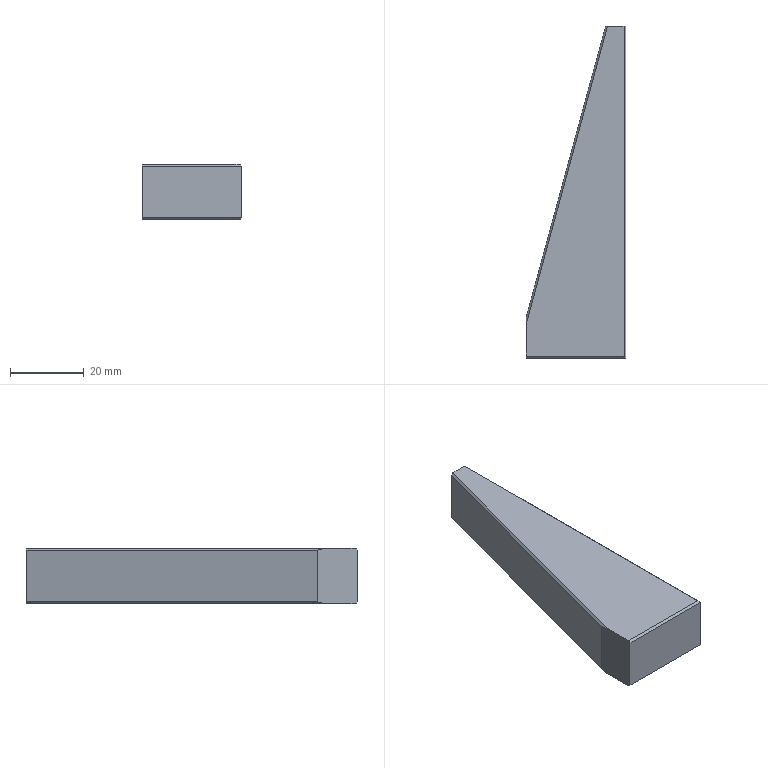Part | SolidWorks | features Chamfer 1, Extrusion 1, ICE 1 | 1 solid | 13 faces | box 27 x 89.833 x 15 mm | volume 23621 mm3 | plane 13
STEP:
#1=CARTESIAN_POINT('',(24.5,89.833,0.5));
#2=VERTEX_POINT('',#1);
#3=CARTESIAN_POINT('',(3.,11.,0.5));
#4=VERTEX_POINT('',#3);
#5=CARTESIAN_POINT('',(30.,110.,0.5));
#6=DIRECTION('',(-0.2631,-0.9648,0.));
#7=VECTOR('',#6,1000.);
#8=LINE('',#5,#7);
#9=EDGE_CURVE('',#2,#4,#8,.T.);
#10=ORIENTED_EDGE('',*,*,#9,.T.);
#11=CARTESIAN_POINT('',(3.,11.,14.5));
#12=VERTEX_POINT('',#11);
#13=CARTESIAN_POINT('',(3.,11.,15.));
#14=DIRECTION('',(0.,0.,1.));
#15=VECTOR('',#14,1000.);
#16=LINE('',#13,#15);
#17=EDGE_CURVE('',#4,#12,#16,.T.);
#18=ORIENTED_EDGE('',*,*,#17,.T.);
#19=CARTESIAN_POINT('',(24.5,89.833,14.5));
#20=VERTEX_POINT('',#19);
#21=CARTESIAN_POINT('',(30.,110.,14.5));
#22=DIRECTION('',(0.2631,0.9648,0.));
#23=VECTOR('',#22,1000.);
#24=LINE('',#21,#23);
#25=EDGE_CURVE('',#12,#20,#24,.T.);
#26=ORIENTED_EDGE('',*,*,#25,.T.);
#27=CARTESIAN_POINT('',(24.5,89.833,0.));
#28=DIRECTION('',(0.,0.,1.));
#29=VECTOR('',#28,1000.);
#30=LINE('',#27,#29);
#31=EDGE_CURVE('',#2,#20,#30,.T.);
#32=ORIENTED_EDGE('',*,*,#31,.F.);
#33=EDGE_LOOP('',(#10,#18,#26,#32));
#34=FACE_OUTER_BOUND('',#33,.T.);
#35=CARTESIAN_POINT('',(30.,110.,15.));
#36=DIRECTION('',(0.9648,-0.2631,0.));
#37=DIRECTION('',(0.2631,0.9648,0.));
#38=AXIS2_PLACEMENT_3D('',#35,#36,#37);
#39=PLANE('',#38);
#40=ADVANCED_FACE('',(#34),#39,.F.);
#41=CARTESIAN_POINT('',(30.,0.,14.5));
#42=VERTEX_POINT('',#41);
#43=CARTESIAN_POINT('',(3.,0.,14.5));
#44=VERTEX_POINT('',#43);
#45=CARTESIAN_POINT('',(0.,0.,14.5));
#46=DIRECTION('',(-1.,0.,0.));
#47=VECTOR('',#46,1000.);
#48=LINE('',#45,#47);
#49=EDGE_CURVE('',#42,#44,#48,.T.);
#50=ORIENTED_EDGE('',*,*,#49,.T.);
#51=CARTESIAN_POINT('',(3.,0.,0.5));
#52=VERTEX_POINT('',#51);
#53=CARTESIAN_POINT('',(3.,0.,0.));
#54=DIRECTION('',(0.,0.,1.));
#55=VECTOR('',#54,1000.);
#56=LINE('',#53,#55);
#57=EDGE_CURVE('',#52,#44,#56,.T.);
#58=ORIENTED_EDGE('',*,*,#57,.F.);
#59=CARTESIAN_POINT('',(30.,0.,0.5));
#60=VERTEX_POINT('',#59);
#61=CARTESIAN_POINT('',(0.,0.,0.5));
#62=DIRECTION('',(1.,0.,0.));
#63=VECTOR('',#62,1000.);
#64=LINE('',#61,#63);
#65=EDGE_CURVE('',#52,#60,#64,.T.);
#66=ORIENTED_EDGE('',*,*,#65,.T.);
#67=CARTESIAN_POINT('',(30.,0.,15.));
#68=DIRECTION('',(0.,0.,-1.));
#69=VECTOR('',#68,1000.);
#70=LINE('',#67,#69);
#71=EDGE_CURVE('',#42,#60,#70,.T.);
#72=ORIENTED_EDGE('',*,*,#71,.F.);
#73=EDGE_LOOP('',(#50,#58,#66,#72));
#74=FACE_OUTER_BOUND('',#73,.T.);
#75=CARTESIAN_POINT('',(0.,0.,15.));
#76=DIRECTION('',(0.,1.,0.));
#77=DIRECTION('',(0.,0.,1.));
#78=AXIS2_PLACEMENT_3D('',#75,#76,#77);
#79=PLANE('',#78);
#80=ADVANCED_FACE('',(#74),#79,.F.);
#81=CARTESIAN_POINT('',(30.,89.833,0.5));
#82=VERTEX_POINT('',#81);
#83=CARTESIAN_POINT('',(30.,0.,0.5));
#84=DIRECTION('',(0.,1.,0.));
#85=VECTOR('',#84,1000.);
#86=LINE('',#83,#85);
#87=EDGE_CURVE('',#60,#82,#86,.T.);
#88=ORIENTED_EDGE('',*,*,#87,.T.);
#89=CARTESIAN_POINT('',(30.,89.833,14.5));
#90=VERTEX_POINT('',#89);
#91=CARTESIAN_POINT('',(30.,89.833,0.));
#92=DIRECTION('',(0.,0.,1.));
#93=VECTOR('',#92,1000.);
#94=LINE('',#91,#93);
#95=EDGE_CURVE('',#82,#90,#94,.T.);
#96=ORIENTED_EDGE('',*,*,#95,.T.);
#97=CARTESIAN_POINT('',(30.,0.,14.5));
#98=DIRECTION('',(0.,-1.,0.));
#99=VECTOR('',#98,1000.);
#100=LINE('',#97,#99);
#101=EDGE_CURVE('',#90,#42,#100,.T.);
#102=ORIENTED_EDGE('',*,*,#101,.T.);
#103=ORIENTED_EDGE('',*,*,#71,.T.);
#104=EDGE_LOOP('',(#88,#96,#102,#103));
#105=FACE_OUTER_BOUND('',#104,.T.);
#106=CARTESIAN_POINT('',(30.,0.,15.));
#107=DIRECTION('',(-1.,0.,0.));
#108=DIRECTION('',(0.,0.,1.));
#109=AXIS2_PLACEMENT_3D('',#106,#107,#108);
#110=PLANE('',#109);
#111=ADVANCED_FACE('',(#105),#110,.F.);
#112=CARTESIAN_POINT('',(3.,0.5,15.));
#113=VERTEX_POINT('',#112);
#114=CARTESIAN_POINT('',(3.,9.1,15.));
#115=VERTEX_POINT('',#114);
#116=CARTESIAN_POINT('',(3.,0.,15.));
#117=DIRECTION('',(0.,1.,0.));
#118=VECTOR('',#117,1000.);
#119=LINE('',#116,#118);
#120=EDGE_CURVE('',#113,#115,#119,.T.);
#121=ORIENTED_EDGE('',*,*,#120,.F.);
#122=CARTESIAN_POINT('',(29.5,0.5,15.));
#123=VERTEX_POINT('',#122);
#124=CARTESIAN_POINT('',(30.,0.5,15.));
#125=DIRECTION('',(1.,0.,0.));
#126=VECTOR('',#125,1000.);
#127=LINE('',#124,#126);
#128=EDGE_CURVE('',#113,#123,#127,.T.);
#129=ORIENTED_EDGE('',*,*,#128,.T.);
#130=CARTESIAN_POINT('',(29.5,89.833,15.));
#131=VERTEX_POINT('',#130);
#132=CARTESIAN_POINT('',(29.5,110.,15.));
#133=DIRECTION('',(0.,1.,0.));
#134=VECTOR('',#133,1000.);
#135=LINE('',#132,#134);
#136=EDGE_CURVE('',#123,#131,#135,.T.);
#137=ORIENTED_EDGE('',*,*,#136,.T.);
#138=CARTESIAN_POINT('',(25.018,89.833,15.));
#139=VERTEX_POINT('',#138);
#140=CARTESIAN_POINT('',(30.,89.833,15.));
#141=DIRECTION('',(1.,0.,0.));
#142=VECTOR('',#141,1000.);
#143=LINE('',#140,#142);
#144=EDGE_CURVE('',#139,#131,#143,.T.);
#145=ORIENTED_EDGE('',*,*,#144,.F.);
#146=CARTESIAN_POINT('',(0.4824,-0.1316,15.));
#147=DIRECTION('',(-0.2631,-0.9648,0.));
#148=VECTOR('',#147,1000.);
#149=LINE('',#146,#148);
#150=EDGE_CURVE('',#139,#115,#149,.T.);
#151=ORIENTED_EDGE('',*,*,#150,.T.);
#152=EDGE_LOOP('',(#121,#129,#137,#145,#151));
#153=FACE_OUTER_BOUND('',#152,.T.);
#154=CARTESIAN_POINT('',(0.,0.,15.));
#155=DIRECTION('',(0.,0.,1.));
#156=DIRECTION('',(1.,0.,0.));
#157=AXIS2_PLACEMENT_3D('',#154,#155,#156);
#158=PLANE('',#157);
#159=ADVANCED_FACE('',(#153),#158,.T.);
#160=CARTESIAN_POINT('',(29.5,0.5,0.));
#161=VERTEX_POINT('',#160);
#162=CARTESIAN_POINT('',(3.,0.5,0.));
#163=VERTEX_POINT('',#162);
#164=CARTESIAN_POINT('',(0.,0.5,0.));
#165=DIRECTION('',(-1.,0.,0.));
#166=VECTOR('',#165,1000.);
#167=LINE('',#164,#166);
#168=EDGE_CURVE('',#161,#163,#167,.T.);
#169=ORIENTED_EDGE('',*,*,#168,.T.);
#170=CARTESIAN_POINT('',(3.,9.1,0.));
#171=VERTEX_POINT('',#170);
#172=CARTESIAN_POINT('',(3.,0.,0.));
#173=DIRECTION('',(0.,1.,0.));
#174=VECTOR('',#173,1000.);
#175=LINE('',#172,#174);
#176=EDGE_CURVE('',#163,#171,#175,.T.);
#177=ORIENTED_EDGE('',*,*,#176,.T.);
#178=CARTESIAN_POINT('',(25.018,89.833,0.));
#179=VERTEX_POINT('',#178);
#180=CARTESIAN_POINT('',(0.4824,-0.1316,0.));
#181=DIRECTION('',(0.2631,0.9648,0.));
#182=VECTOR('',#181,1000.);
#183=LINE('',#180,#182);
#184=EDGE_CURVE('',#171,#179,#183,.T.);
#185=ORIENTED_EDGE('',*,*,#184,.T.);
#186=CARTESIAN_POINT('',(29.5,89.833,0.));
#187=VERTEX_POINT('',#186);
#188=CARTESIAN_POINT('',(30.,89.833,0.));
#189=DIRECTION('',(1.,0.,0.));
#190=VECTOR('',#189,1000.);
#191=LINE('',#188,#190);
#192=EDGE_CURVE('',#179,#187,#191,.T.);
#193=ORIENTED_EDGE('',*,*,#192,.T.);
#194=CARTESIAN_POINT('',(29.5,0.,0.));
#195=DIRECTION('',(0.,-1.,0.));
#196=VECTOR('',#195,1000.);
#197=LINE('',#194,#196);
#198=EDGE_CURVE('',#187,#161,#197,.T.);
#199=ORIENTED_EDGE('',*,*,#198,.T.);
#200=EDGE_LOOP('',(#169,#177,#185,#193,#199));
#201=FACE_OUTER_BOUND('',#200,.T.);
#202=CARTESIAN_POINT('',(0.,0.,0.));
#203=DIRECTION('',(0.,0.,1.));
#204=DIRECTION('',(1.,0.,0.));
#205=AXIS2_PLACEMENT_3D('',#202,#203,#204);
#206=PLANE('',#205);
#207=ADVANCED_FACE('',(#201),#206,.F.);
#208=CARTESIAN_POINT('',(3.,103.59,24.862));
#209=DIRECTION('',(0.,-0.9671,-0.2545));
#210=VECTOR('',#209,1000.);
#211=LINE('',#208,#210);
#212=EDGE_CURVE('',#4,#171,#211,.T.);
#213=ORIENTED_EDGE('',*,*,#212,.F.);
#214=ORIENTED_EDGE('',*,*,#9,.F.);
#215=CARTESIAN_POINT('',(27.349,89.833,-2.248));
#216=DIRECTION('',(-0.7197,0.,0.6943));
#217=VECTOR('',#216,1000.);
#218=LINE('',#215,#217);
#219=EDGE_CURVE('',#179,#2,#218,.T.);
#220=ORIENTED_EDGE('',*,*,#219,.F.);
#221=ORIENTED_EDGE('',*,*,#184,.F.);
#222=EDGE_LOOP('',(#213,#214,#220,#221));
#223=FACE_OUTER_BOUND('',#222,.T.);
#224=CARTESIAN_POINT('',(30.,110.,0.5));
#225=DIRECTION('',(0.6822,-0.1861,0.7071));
#226=DIRECTION('',(-0.2631,-0.9648,0.));
#227=AXIS2_PLACEMENT_3D('',#224,#225,#226);
#228=PLANE('',#227);
#229=ADVANCED_FACE('',(#223),#228,.F.);
#230=CARTESIAN_POINT('',(30.,89.833,0.5));
#231=DIRECTION('',(-0.7071,0.,-0.7071));
#232=VECTOR('',#231,1000.);
#233=LINE('',#230,#232);
#234=EDGE_CURVE('',#82,#187,#233,.T.);
#235=ORIENTED_EDGE('',*,*,#234,.F.);
#236=ORIENTED_EDGE('',*,*,#87,.F.);
#237=CARTESIAN_POINT('',(30.,0.,0.5));
#238=DIRECTION('',(0.5774,-0.5774,0.5774));
#239=VECTOR('',#238,1000.);
#240=LINE('',#237,#239);
#241=EDGE_CURVE('',#161,#60,#240,.T.);
#242=ORIENTED_EDGE('',*,*,#241,.F.);
#243=ORIENTED_EDGE('',*,*,#198,.F.);
#244=EDGE_LOOP('',(#235,#236,#242,#243));
#245=FACE_OUTER_BOUND('',#244,.T.);
#246=CARTESIAN_POINT('',(30.,0.,0.5));
#247=DIRECTION('',(-0.7071,0.,0.7071));
#248=DIRECTION('',(0.,1.,0.));
#249=AXIS2_PLACEMENT_3D('',#246,#247,#248);
#250=PLANE('',#249);
#251=ADVANCED_FACE('',(#245),#250,.F.);
#252=CARTESIAN_POINT('',(3.,0.,0.5));
#253=DIRECTION('',(0.,-0.7071,0.7071));
#254=VECTOR('',#253,1000.);
#255=LINE('',#252,#254);
#256=EDGE_CURVE('',#163,#52,#255,.T.);
#257=ORIENTED_EDGE('',*,*,#256,.F.);
#258=ORIENTED_EDGE('',*,*,#168,.F.);
#259=ORIENTED_EDGE('',*,*,#241,.T.);
#260=ORIENTED_EDGE('',*,*,#65,.F.);
#261=EDGE_LOOP('',(#257,#258,#259,#260));
#262=FACE_OUTER_BOUND('',#261,.T.);
#263=CARTESIAN_POINT('',(0.,0.,0.5));
#264=DIRECTION('',(0.,0.7071,0.7071));
#265=DIRECTION('',(1.,0.,0.));
#266=AXIS2_PLACEMENT_3D('',#263,#264,#265);
#267=PLANE('',#266);
#268=ADVANCED_FACE('',(#262),#267,.F.);
#269=CARTESIAN_POINT('',(3.,0.5,15.));
#270=DIRECTION('',(0.,0.7071,0.7071));
#271=VECTOR('',#270,1000.);
#272=LINE('',#269,#271);
#273=EDGE_CURVE('',#44,#113,#272,.T.);
#274=ORIENTED_EDGE('',*,*,#273,.F.);
#275=ORIENTED_EDGE('',*,*,#49,.F.);
#276=CARTESIAN_POINT('',(19.667,10.333,24.833));
#277=DIRECTION('',(0.5774,-0.5774,-0.5774));
#278=VECTOR('',#277,1000.);
#279=LINE('',#276,#278);
#280=EDGE_CURVE('',#123,#42,#279,.T.);
#281=ORIENTED_EDGE('',*,*,#280,.F.);
#282=ORIENTED_EDGE('',*,*,#128,.F.);
#283=EDGE_LOOP('',(#274,#275,#281,#282));
#284=FACE_OUTER_BOUND('',#283,.T.);
#285=CARTESIAN_POINT('',(0.,0.5,15.));
#286=DIRECTION('',(0.,-0.7071,0.7071));
#287=DIRECTION('',(-1.,0.,0.));
#288=AXIS2_PLACEMENT_3D('',#285,#286,#287);
#289=PLANE('',#288);
#290=ADVANCED_FACE('',(#284),#289,.T.);
#291=CARTESIAN_POINT('',(3.,0.4661,17.272));
#292=DIRECTION('',(0.,0.9671,-0.2545));
#293=VECTOR('',#292,1000.);
#294=LINE('',#291,#293);
#295=EDGE_CURVE('',#115,#12,#294,.T.);
#296=ORIENTED_EDGE('',*,*,#295,.F.);
#297=ORIENTED_EDGE('',*,*,#150,.F.);
#298=CARTESIAN_POINT('',(12.31,89.833,2.74));
#299=DIRECTION('',(0.7197,0.,0.6943));
#300=VECTOR('',#299,1000.);
#301=LINE('',#298,#300);
#302=EDGE_CURVE('',#20,#139,#301,.T.);
#303=ORIENTED_EDGE('',*,*,#302,.F.);
#304=ORIENTED_EDGE('',*,*,#25,.F.);
#305=EDGE_LOOP('',(#296,#297,#303,#304));
#306=FACE_OUTER_BOUND('',#305,.T.);
#307=CARTESIAN_POINT('',(0.4824,-0.1316,15.));
#308=DIRECTION('',(-0.6822,0.1861,0.7071));
#309=DIRECTION('',(0.2631,0.9648,0.));
#310=AXIS2_PLACEMENT_3D('',#307,#308,#309);
#311=PLANE('',#310);
#312=ADVANCED_FACE('',(#306),#311,.T.);
#313=CARTESIAN_POINT('',(29.5,89.833,15.));
#314=DIRECTION('',(0.7071,0.,-0.7071));
#315=VECTOR('',#314,1000.);
#316=LINE('',#313,#315);
#317=EDGE_CURVE('',#131,#90,#316,.T.);
#318=ORIENTED_EDGE('',*,*,#317,.F.);
#319=ORIENTED_EDGE('',*,*,#136,.F.);
#320=ORIENTED_EDGE('',*,*,#280,.T.);
#321=ORIENTED_EDGE('',*,*,#101,.F.);
#322=EDGE_LOOP('',(#318,#319,#320,#321));
#323=FACE_OUTER_BOUND('',#322,.T.);
#324=CARTESIAN_POINT('',(29.5,0.,15.));
#325=DIRECTION('',(0.7071,0.,0.7071));
#326=DIRECTION('',(0.,-1.,0.));
#327=AXIS2_PLACEMENT_3D('',#324,#325,#326);
#328=PLANE('',#327);
#329=ADVANCED_FACE('',(#323),#328,.T.);
#330=ORIENTED_EDGE('',*,*,#219,.T.);
#331=ORIENTED_EDGE('',*,*,#31,.T.);
#332=ORIENTED_EDGE('',*,*,#302,.T.);
#333=ORIENTED_EDGE('',*,*,#144,.T.);
#334=ORIENTED_EDGE('',*,*,#317,.T.);
#335=ORIENTED_EDGE('',*,*,#95,.F.);
#336=ORIENTED_EDGE('',*,*,#234,.T.);
#337=ORIENTED_EDGE('',*,*,#192,.F.);
#338=EDGE_LOOP('',(#330,#331,#332,#333,#334,#335,#336,#337));
#339=FACE_OUTER_BOUND('',#338,.T.);
#340=CARTESIAN_POINT('',(30.,89.833,0.));
#341=DIRECTION('',(0.,-1.,0.));
#342=DIRECTION('',(0.,0.,-1.));
#343=AXIS2_PLACEMENT_3D('',#340,#341,#342);
#344=PLANE('',#343);
#345=ADVANCED_FACE('',(#339),#344,.F.);
#346=ORIENTED_EDGE('',*,*,#256,.T.);
#347=ORIENTED_EDGE('',*,*,#57,.T.);
#348=ORIENTED_EDGE('',*,*,#273,.T.);
#349=ORIENTED_EDGE('',*,*,#120,.T.);
#350=ORIENTED_EDGE('',*,*,#295,.T.);
#351=ORIENTED_EDGE('',*,*,#17,.F.);
#352=ORIENTED_EDGE('',*,*,#212,.T.);
#353=ORIENTED_EDGE('',*,*,#176,.F.);
#354=EDGE_LOOP('',(#346,#347,#348,#349,#350,#351,#352,#353));
#355=FACE_OUTER_BOUND('',#354,.T.);
#356=CARTESIAN_POINT('',(3.,0.,0.));
#357=DIRECTION('',(1.,0.,0.));
#358=DIRECTION('',(0.,0.,-1.));
#359=AXIS2_PLACEMENT_3D('',#356,#357,#358);
#360=PLANE('',#359);
#361=ADVANCED_FACE('',(#355),#360,.F.);
#362=CLOSED_SHELL('',(#40,#80,#111,#159,#207,#229,#251,#268,#290,#312,#329,#345,#361));
#363=MANIFOLD_SOLID_BREP('',#362);
#364=CARTESIAN_POINT('',(0.,0.,0.));
#365=DIRECTION('',(0.,0.,1.));
#366=DIRECTION('',(1.,0.,0.));
#367=AXIS2_PLACEMENT_3D('',#364,#365,#366);
#368=(LENGTH_UNIT()NAMED_UNIT(*)SI_UNIT(.MILLI.,.METRE.));
#369=UNCERTAINTY_MEASURE_WITH_UNIT(LENGTH_MEASURE(0.00001),#368,'','');
#370=(NAMED_UNIT(*)PLANE_ANGLE_UNIT()SI_UNIT($,.RADIAN.));
#371=(NAMED_UNIT(*)SI_UNIT($,.STERADIAN.)SOLID_ANGLE_UNIT());
#372=(GEOMETRIC_REPRESENTATION_CONTEXT(3)GLOBAL_UNCERTAINTY_ASSIGNED_CONTEXT((#369))GLOBAL_UNIT_ASSIGNED_CONTEXT((#368,#370,#371))REPRESENTATION_CONTEXT('',''));
#373=ADVANCED_BREP_SHAPE_REPRESENTATION('',(#363,#367),#372);